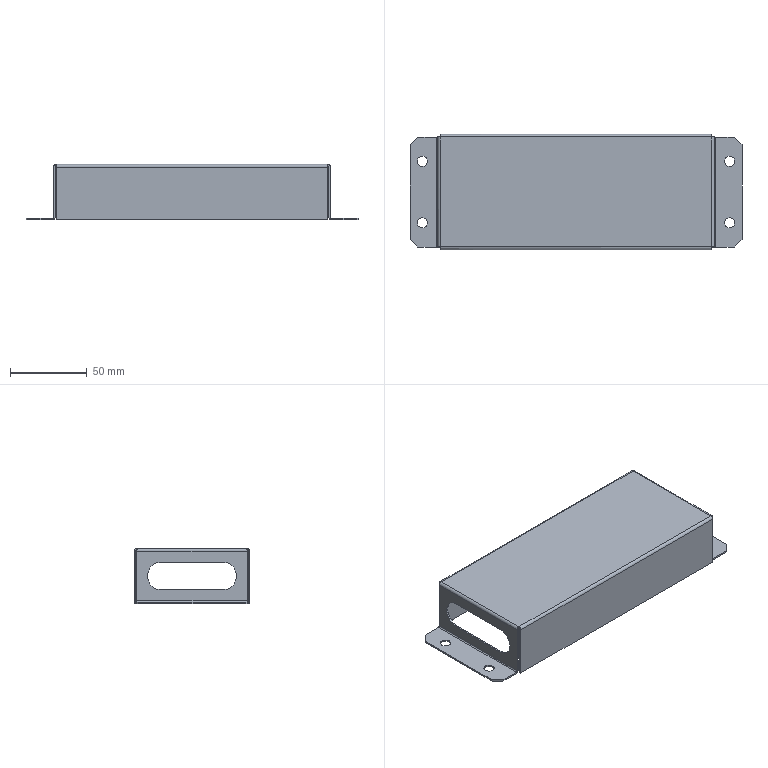Part | NX | 1 solid | 70 faces | box 216 x 75 x 36 mm | volume 30962 mm3 | plane 42 | cylinder 20 | spline 8 | commonest cylinder face diameters 1.473 x6 3.473 x6 6.6 x4 18 x4